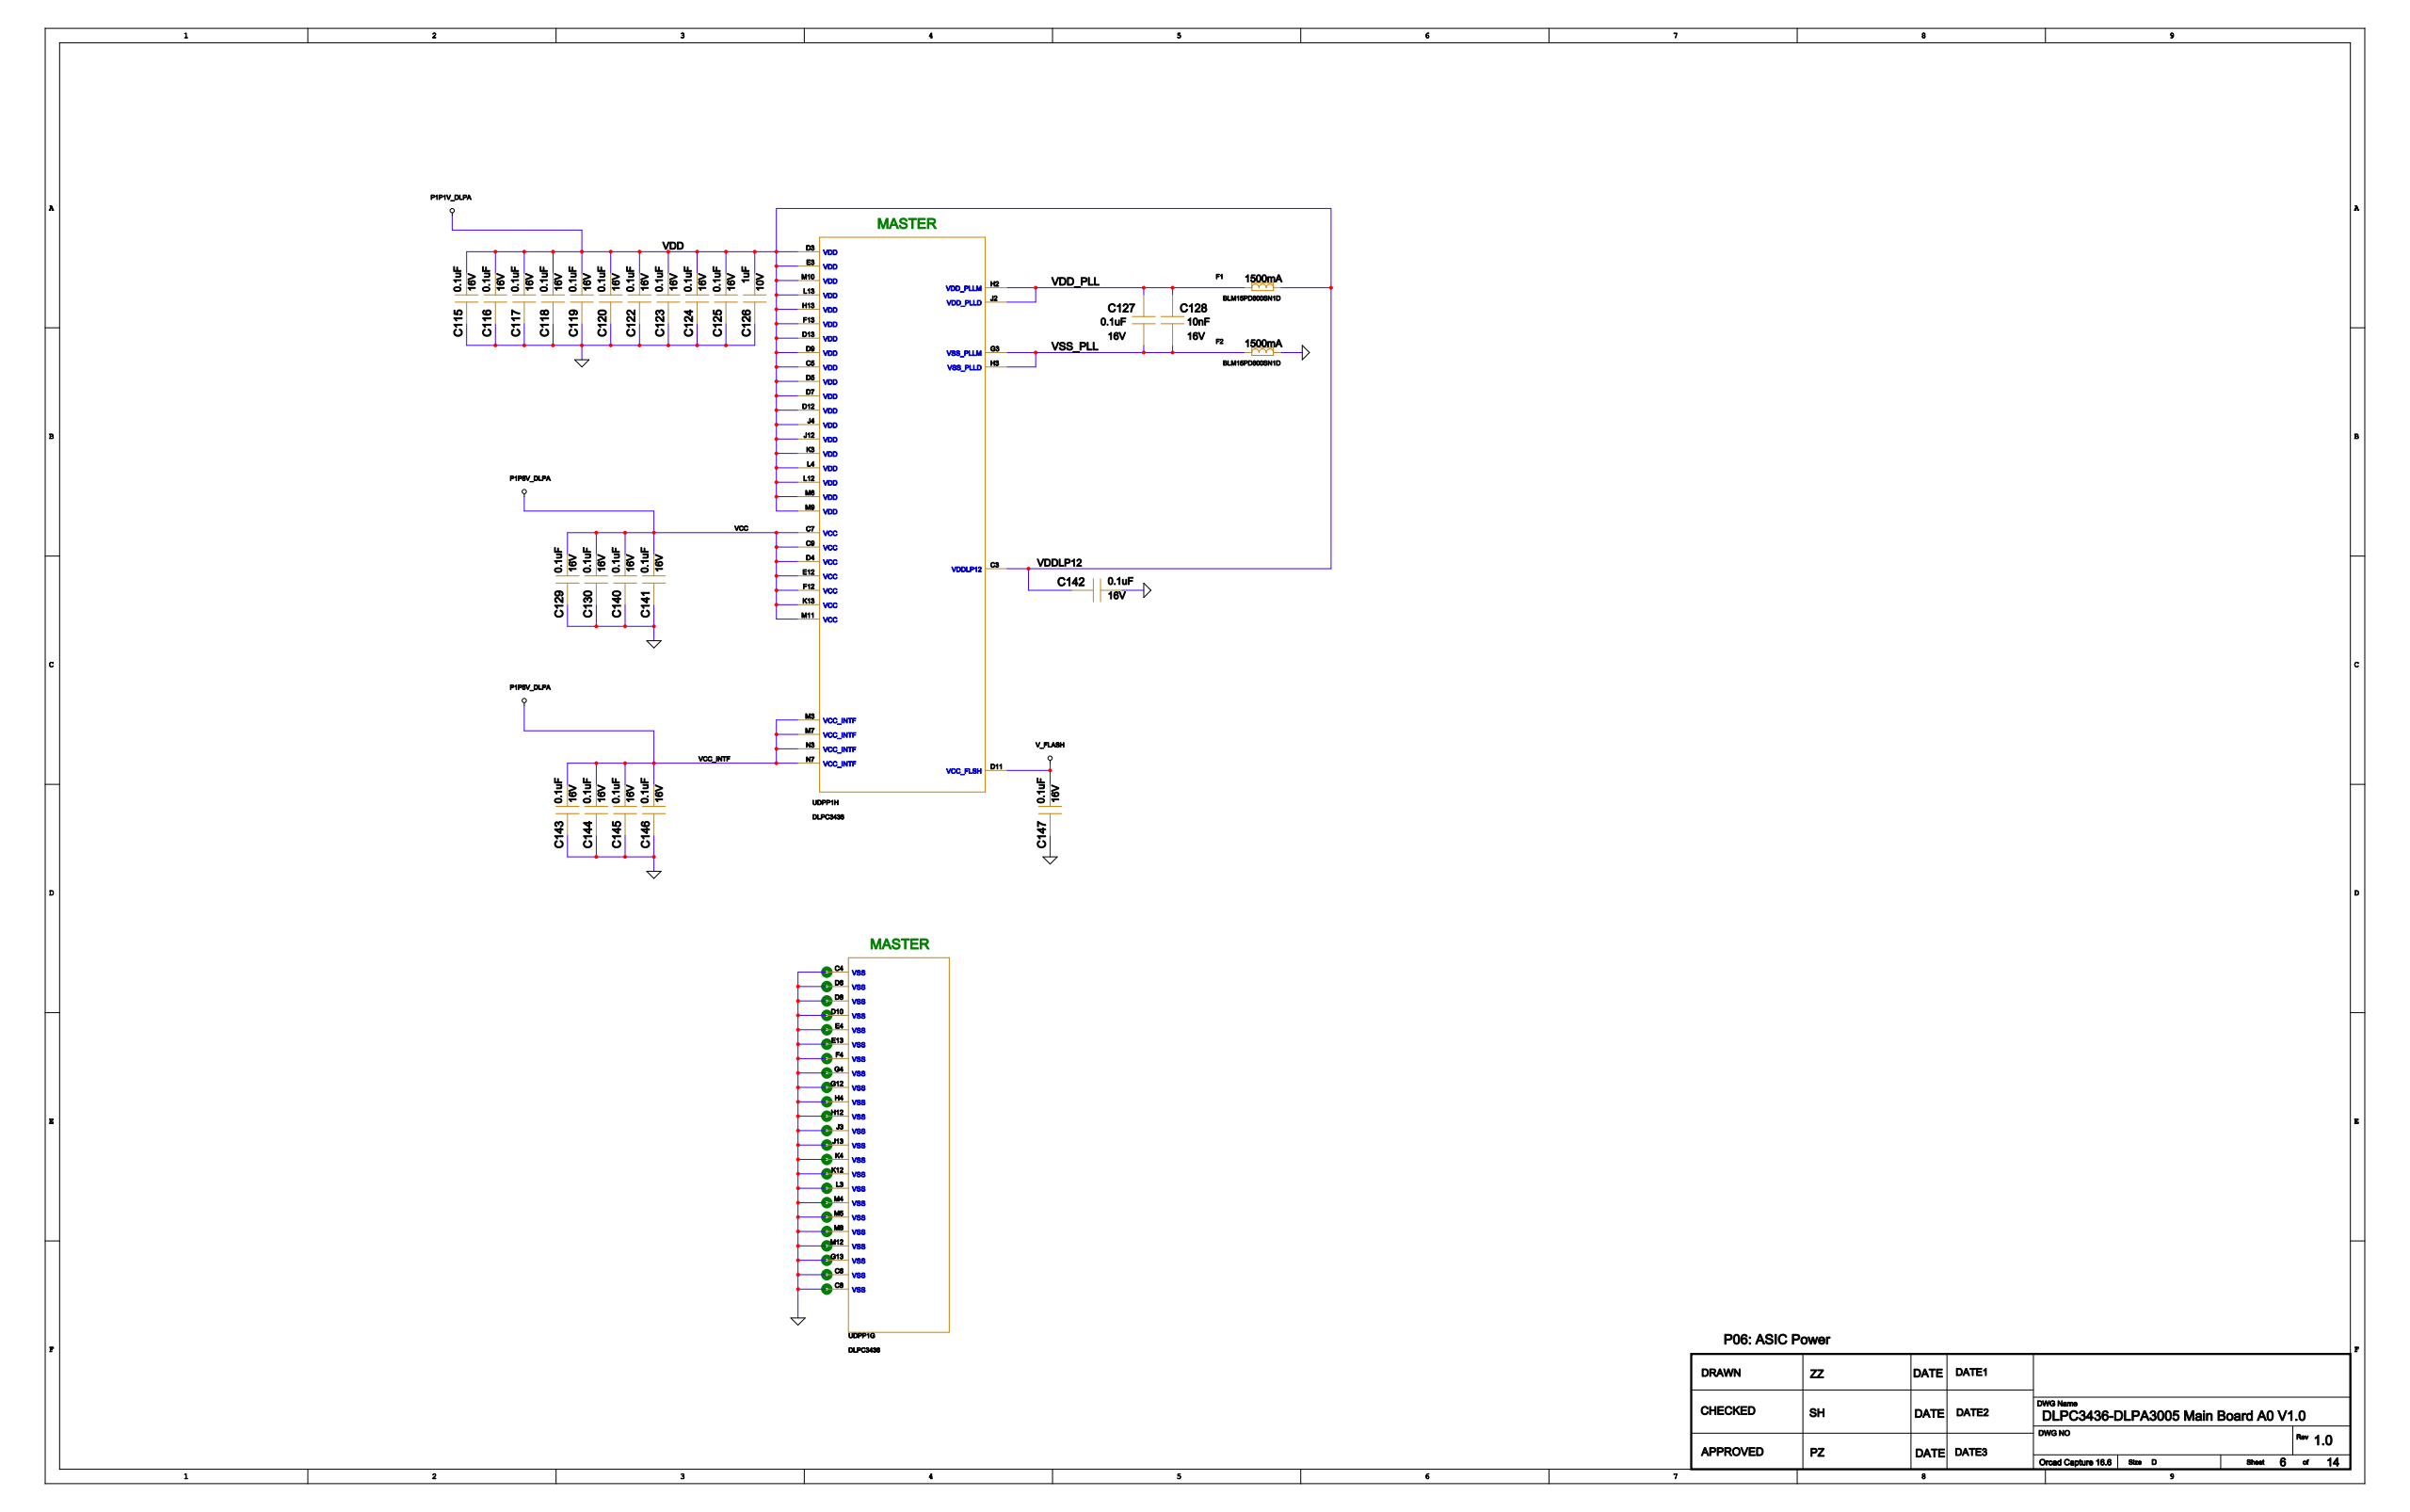Circuit board | Cadence Allegro | 1223 parts | 777 nets | one sheet of the schematic
Parts on this sheet (reference | value | footprint):
C115 | 0.1uF | C0201
C116 | 0.1uF | C0201
C117 | 0.1uF | C0201
C118 | 0.1uF | C0201
C119 | 0.1uF | C0201
C120 | 0.1uF | C0201
C122 | 0.1uF | C0201
C123 | 0.1uF | C0201
C124 | 0.1uF | C0201
C125 | 0.1uF | C0201
C126 | 1uF | C0402
C127 | 0.1uF | C0201
C128 | 10nF | C0201
C129 | 0.1uF | C0201
C130 | 0.1uF | C0201
C140 | 0.1uF | C0201
C141 | 0.1uF | C0201
C142 | 0.1uF | C0201
C143 | 0.1uF | C0201
C144 | 0.1uF | C0201
C145 | 0.1uF | C0201
C146 | 0.1uF | C0201
C147 | 0.1uF | C0201
F1 | BLM15PD800SN1D | R0402
F2 | BLM15PD800SN1D | R0402
UDPP1 | DLPC3436 | DLPC3436_176NFBGA
Nets of these parts (net: part-pin ...):
GND: C115-2 C116-2 C117-2 C118-2 C119-2 C120-2 C122-2 C123-2 C124-2 C125-2 C126-2 C129-2 C130-2 C140-2 C141-2 C142-2 C143-2 C144-2 C145-2 C146-2 C147-2 F2-2 UDPP1-C4 UDPP1-C6 UDPP1-C8 UDPP1-D6 UDPP1-D8 UDPP1-D10 UDPP1-E4 UDPP1-E13 UDPP1-F4 UDPP1-G4 UDPP1-G12 UDPP1-G13 UDPP1-H4 UDPP1-H12 UDPP1-J3 UDPP1-J13 UDPP1-K4 UDPP1-K12 UDPP1-L3 UDPP1-M4 UDPP1-M5 UDPP1-M8 UDPP1-M12
P1P8V_DLPA: C129-1 C130-1 C140-1 C141-1 C143-1 C144-1 C145-1 C146-1 UDPP1-C7 UDPP1-C9 UDPP1-D4 UDPP1-E12 UDPP1-F12 UDPP1-K13 UDPP1-M3 UDPP1-M7 UDPP1-M11 UDPP1-N3 UDPP1-N7
V_FLASH: C147-1 UDPP1-D11
P1P1V_DLPA: C115-1 C116-1 C117-1 C118-1 C119-1 C120-1 C122-1 C123-1 C124-1 C125-1 C126-1 C142-1 F1-2 UDPP1-C3 UDPP1-C5 UDPP1-D3 UDPP1-D5 UDPP1-D7 UDPP1-D9 UDPP1-D12 UDPP1-D13 UDPP1-E3 UDPP1-F13 UDPP1-H13 UDPP1-J4 UDPP1-J12 UDPP1-K3 UDPP1-L4 UDPP1-L12 UDPP1-L13 UDPP1-M6 UDPP1-M9 UDPP1-M10
VSS_PLL: C127-2 C128-1 F2-1 UDPP1-G3 UDPP1-H3
VDD_PLL: C127-1 C128-2 F1-1 UDPP1-H2 UDPP1-J2